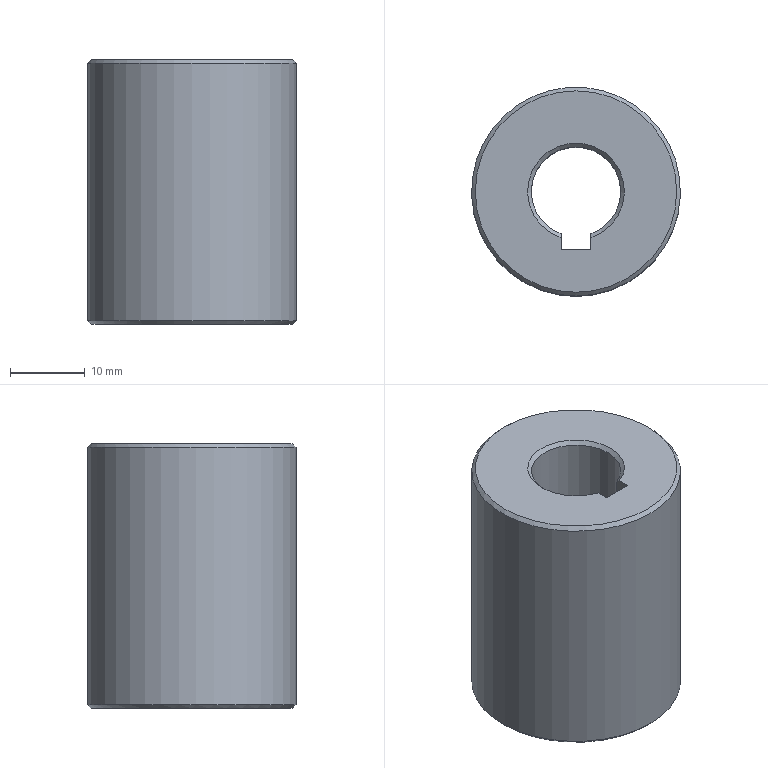Part | STEP file | 1 solid | 17 faces | box 28 x 28 x 35.5 mm | volume 17370 mm3 | cone 8 | plane 5 | cylinder 4 | commonest cylinder face diameters 3.242 x2 12 x1 28 x1
STEP:
#1=CARTESIAN_POINT('',(0.,0.,0.));
#2=DIRECTION('',(0.,0.,1.));
#3=DIRECTION('',(1.,0.,0.));
#4=AXIS2_PLACEMENT_3D('',#1,#2,#3);
#5=CARTESIAN_POINT('',(0.,-14.,0.5));
#6=VERTEX_POINT('',#5);
#7=CARTESIAN_POINT('',(0.,0.,0.5));
#8=DIRECTION('',(0.,0.,1.));
#9=DIRECTION('',(1.,0.,0.));
#10=AXIS2_PLACEMENT_3D('',#7,#8,#9);
#11=CIRCLE('',#10,14.);
#12=CARTESIAN_POINT('',(0.,0.,0.5));
#13=DIRECTION('',(0.,0.,1.));
#14=DIRECTION('',(0.,1.,0.));
#15=AXIS2_PLACEMENT_3D('',#12,#13,#14);
#16=CONICAL_SURFACE('',#15,14.,0.7854);
#17=CARTESIAN_POINT('',(-1.571,0.));
#18=DIRECTION('',(1.,0.));
#19=VECTOR('',#18,1.);
#20=LINE('',#17,#19);
#21=(GEOMETRIC_REPRESENTATION_CONTEXT(2)PARAMETRIC_REPRESENTATION_CONTEXT()REPRESENTATION_CONTEXT('',''));
#22=DEFINITIONAL_REPRESENTATION('',(#20),#21);
#23=PCURVE('',#16,#22);
#24=CARTESIAN_POINT('',(0.,0.,17.75));
#25=DIRECTION('',(0.,0.,-1.));
#26=DIRECTION('',(0.,-1.,0.));
#27=AXIS2_PLACEMENT_3D('',#24,#25,#26);
#28=CYLINDRICAL_SURFACE('',#27,14.);
#29=CARTESIAN_POINT('',(10.996,17.25));
#30=DIRECTION('',(-1.,0.));
#31=VECTOR('',#30,1.);
#32=LINE('',#29,#31);
#33=(GEOMETRIC_REPRESENTATION_CONTEXT(2)PARAMETRIC_REPRESENTATION_CONTEXT()REPRESENTATION_CONTEXT('',''));
#34=DEFINITIONAL_REPRESENTATION('',(#32),#33);
#35=PCURVE('',#28,#34);
#36=SURFACE_CURVE('',#11,(#23,#35),.PCURVE_S1.);
#37=EDGE_CURVE('',#6,#6,#36,.T.);
#38=ORIENTED_EDGE('',*,*,#37,.F.);
#39=CARTESIAN_POINT('',(0.,-13.5,0.));
#40=VERTEX_POINT('',#39);
#41=CARTESIAN_POINT('',(0.,-13.5,0.));
#42=CARTESIAN_POINT('',(0.,-14.,0.5));
#43=B_SPLINE_CURVE_WITH_KNOTS('',1,(#41,#42),.UNSPECIFIED.,.F.,.F.,(2,2),(-0.7071,0.),.PIECEWISE_BEZIER_KNOTS.);
#44=CARTESIAN_POINT('',(3.142,0.));
#45=DIRECTION('',(0.,1.));
#46=VECTOR('',#45,1.);
#47=LINE('',#44,#46);
#48=(GEOMETRIC_REPRESENTATION_CONTEXT(2)PARAMETRIC_REPRESENTATION_CONTEXT()REPRESENTATION_CONTEXT('',''));
#49=DEFINITIONAL_REPRESENTATION('',(#47),#48);
#50=PCURVE('',#16,#49);
#51=CARTESIAN_POINT('',(9.425,0.));
#52=DIRECTION('',(0.,1.));
#53=VECTOR('',#52,1.);
#54=LINE('',#51,#53);
#55=(GEOMETRIC_REPRESENTATION_CONTEXT(2)PARAMETRIC_REPRESENTATION_CONTEXT()REPRESENTATION_CONTEXT('',''));
#56=DEFINITIONAL_REPRESENTATION('',(#54),#55);
#57=PCURVE('',#16,#56);
#58=SEAM_CURVE('',#43,(#50,#57),.PCURVE_S1.);
#59=EDGE_CURVE('',#40,#6,#58,.T.);
#60=ORIENTED_EDGE('',*,*,#59,.F.);
#61=CARTESIAN_POINT('',(0.,0.,0.));
#62=DIRECTION('',(0.,0.,1.));
#63=DIRECTION('',(1.,0.,0.));
#64=AXIS2_PLACEMENT_3D('',#61,#62,#63);
#65=CIRCLE('',#64,13.5);
#66=CARTESIAN_POINT('',(-1.571,-0.5));
#67=DIRECTION('',(1.,0.));
#68=VECTOR('',#67,1.);
#69=LINE('',#66,#68);
#70=(GEOMETRIC_REPRESENTATION_CONTEXT(2)PARAMETRIC_REPRESENTATION_CONTEXT()REPRESENTATION_CONTEXT('',''));
#71=DEFINITIONAL_REPRESENTATION('',(#69),#70);
#72=PCURVE('',#16,#71);
#73=CARTESIAN_POINT('',(0.,10.,0.));
#74=DIRECTION('',(0.,0.,1.));
#75=DIRECTION('',(1.,0.,0.));
#76=AXIS2_PLACEMENT_3D('',#73,#74,#75);
#77=PLANE('',#76);
#78=CARTESIAN_POINT('',(0.,-10.));
#79=DIRECTION('',(1.,0.));
#80=AXIS2_PLACEMENT_2D('',#78,#79);
#81=CIRCLE('',#80,13.5);
#82=(GEOMETRIC_REPRESENTATION_CONTEXT(2)PARAMETRIC_REPRESENTATION_CONTEXT()REPRESENTATION_CONTEXT('',''));
#83=DEFINITIONAL_REPRESENTATION('',(#81),#82);
#84=PCURVE('',#77,#83);
#85=SURFACE_CURVE('',#65,(#72,#84),.PCURVE_S1.);
#86=EDGE_CURVE('',#40,#40,#85,.T.);
#87=ORIENTED_EDGE('',*,*,#86,.T.);
#88=ORIENTED_EDGE('',*,*,#59,.T.);
#89=EDGE_LOOP('',(#38,#60,#87,#88));
#90=FACE_BOUND('',#89,.T.);
#91=ADVANCED_FACE('',(#90),#16,.T.);
#92=CARTESIAN_POINT('',(0.,-14.,35.));
#93=VERTEX_POINT('',#92);
#94=CARTESIAN_POINT('',(0.,0.,35.));
#95=DIRECTION('',(0.,0.,-1.));
#96=DIRECTION('',(1.,0.,0.));
#97=AXIS2_PLACEMENT_3D('',#94,#95,#96);
#98=CIRCLE('',#97,14.);
#99=CARTESIAN_POINT('',(-1.571,-17.25));
#100=DIRECTION('',(1.,0.));
#101=VECTOR('',#100,1.);
#102=LINE('',#99,#101);
#103=(GEOMETRIC_REPRESENTATION_CONTEXT(2)PARAMETRIC_REPRESENTATION_CONTEXT()REPRESENTATION_CONTEXT('',''));
#104=DEFINITIONAL_REPRESENTATION('',(#102),#103);
#105=PCURVE('',#28,#104);
#106=CARTESIAN_POINT('',(0.,0.,35.));
#107=DIRECTION('',(0.,0.,-1.));
#108=DIRECTION('',(0.,-1.,0.));
#109=AXIS2_PLACEMENT_3D('',#106,#107,#108);
#110=CONICAL_SURFACE('',#109,14.,0.7854);
#111=CARTESIAN_POINT('',(-1.571,0.));
#112=DIRECTION('',(1.,0.));
#113=VECTOR('',#112,1.);
#114=LINE('',#111,#113);
#115=(GEOMETRIC_REPRESENTATION_CONTEXT(2)PARAMETRIC_REPRESENTATION_CONTEXT()REPRESENTATION_CONTEXT('',''));
#116=DEFINITIONAL_REPRESENTATION('',(#114),#115);
#117=PCURVE('',#110,#116);
#118=SURFACE_CURVE('',#98,(#105,#117),.PCURVE_S1.);
#119=EDGE_CURVE('',#93,#93,#118,.T.);
#120=ORIENTED_EDGE('',*,*,#119,.T.);
#121=CARTESIAN_POINT('',(0.,-14.,35.));
#122=CARTESIAN_POINT('',(0.,-14.,0.5));
#123=B_SPLINE_CURVE_WITH_KNOTS('',1,(#121,#122),.UNSPECIFIED.,.F.,.F.,(2,2),(-17.25,17.25),.PIECEWISE_BEZIER_KNOTS.);
#124=CARTESIAN_POINT('',(6.283,0.));
#125=DIRECTION('',(0.,1.));
#126=VECTOR('',#125,1.);
#127=LINE('',#124,#126);
#128=(GEOMETRIC_REPRESENTATION_CONTEXT(2)PARAMETRIC_REPRESENTATION_CONTEXT()REPRESENTATION_CONTEXT('',''));
#129=DEFINITIONAL_REPRESENTATION('',(#127),#128);
#130=PCURVE('',#28,#129);
#131=CARTESIAN_POINT('',(0.,0.));
#132=DIRECTION('',(0.,1.));
#133=VECTOR('',#132,1.);
#134=LINE('',#131,#133);
#135=(GEOMETRIC_REPRESENTATION_CONTEXT(2)PARAMETRIC_REPRESENTATION_CONTEXT()REPRESENTATION_CONTEXT('',''));
#136=DEFINITIONAL_REPRESENTATION('',(#134),#135);
#137=PCURVE('',#28,#136);
#138=SEAM_CURVE('',#123,(#130,#137),.PCURVE_S1.);
#139=EDGE_CURVE('',#93,#6,#138,.T.);
#140=ORIENTED_EDGE('',*,*,#139,.T.);
#141=ORIENTED_EDGE('',*,*,#37,.T.);
#142=ORIENTED_EDGE('',*,*,#139,.F.);
#143=EDGE_LOOP('',(#120,#140,#141,#142));
#144=FACE_BOUND('',#143,.T.);
#145=ADVANCED_FACE('',(#144),#28,.T.);
#146=ORIENTED_EDGE('',*,*,#86,.F.);
#147=EDGE_LOOP('',(#146));
#148=FACE_BOUND('',#147,.T.);
#149=CARTESIAN_POINT('',(-2.,-6.185,0.));
#150=VERTEX_POINT('',#149);
#151=CARTESIAN_POINT('',(2.,-6.185,0.));
#152=VERTEX_POINT('',#151);
#153=CARTESIAN_POINT('',(0.,0.,0.));
#154=DIRECTION('',(0.,0.,-1.));
#155=DIRECTION('',(0.3077,-0.9515,0.));
#156=AXIS2_PLACEMENT_3D('',#153,#154,#155);
#157=CIRCLE('',#156,6.5);
#158=CARTESIAN_POINT('',(2.,-16.185));
#159=CARTESIAN_POINT('',(-8.712,-19.649));
#160=CARTESIAN_POINT('',(-6.356,-8.64));
#161=CARTESIAN_POINT('',(-4.,2.369));
#162=CARTESIAN_POINT('',(4.356,-5.176));
#163=CARTESIAN_POINT('',(12.712,-12.721));
#164=CARTESIAN_POINT('',(2.,-16.185));
#165=(BOUNDED_CURVE()B_SPLINE_CURVE(2,(#158,#159,#160,#161,#162,#163,#164),.UNSPECIFIED.,.T.,.F.)B_SPLINE_CURVE_WITH_KNOTS((1,2,2,2,2,1),(-2.094,0.,2.094,4.189,6.283,8.378),.UNSPECIFIED.)CURVE()GEOMETRIC_REPRESENTATION_ITEM()RATIONAL_B_SPLINE_CURVE((1.,0.5,1.,0.5,1.,0.5,1.))REPRESENTATION_ITEM(''));
#166=(GEOMETRIC_REPRESENTATION_CONTEXT(2)PARAMETRIC_REPRESENTATION_CONTEXT()REPRESENTATION_CONTEXT('',''));
#167=DEFINITIONAL_REPRESENTATION('',(#165),#166);
#168=PCURVE('',#77,#167);
#169=CARTESIAN_POINT('',(0.,0.,0.));
#170=DIRECTION('',(0.,0.,-1.));
#171=DIRECTION('',(0.,1.,0.));
#172=AXIS2_PLACEMENT_3D('',#169,#170,#171);
#173=CONICAL_SURFACE('',#172,6.5,0.7854);
#174=CARTESIAN_POINT('',(-3.454,0.));
#175=DIRECTION('',(1.,0.));
#176=VECTOR('',#175,1.);
#177=LINE('',#174,#176);
#178=(GEOMETRIC_REPRESENTATION_CONTEXT(2)PARAMETRIC_REPRESENTATION_CONTEXT()REPRESENTATION_CONTEXT('',''));
#179=DEFINITIONAL_REPRESENTATION('',(#177),#178);
#180=PCURVE('',#173,#179);
#181=SURFACE_CURVE('',#157,(#168,#180),.PCURVE_S1.);
#182=EDGE_CURVE('',#150,#152,#181,.T.);
#183=ORIENTED_EDGE('',*,*,#182,.F.);
#184=CARTESIAN_POINT('',(-2.,-7.8,0.));
#185=VERTEX_POINT('',#184);
#186=CARTESIAN_POINT('',(-2.,-6.185,0.));
#187=DIRECTION('',(0.,-1.,0.));
#188=VECTOR('',#187,1.);
#189=LINE('',#186,#188);
#190=CARTESIAN_POINT('',(-2.,-16.185));
#191=DIRECTION('',(0.,-1.));
#192=VECTOR('',#191,1.);
#193=LINE('',#190,#192);
#194=(GEOMETRIC_REPRESENTATION_CONTEXT(2)PARAMETRIC_REPRESENTATION_CONTEXT()REPRESENTATION_CONTEXT('',''));
#195=DEFINITIONAL_REPRESENTATION('',(#193),#194);
#196=PCURVE('',#77,#195);
#197=CARTESIAN_POINT('',(-2.,-7.8,0.));
#198=DIRECTION('',(-1.,0.,0.));
#199=DIRECTION('',(0.,0.,1.));
#200=AXIS2_PLACEMENT_3D('',#197,#198,#199);
#201=PLANE('',#200);
#202=CARTESIAN_POINT('',(0.,1.615));
#203=DIRECTION('',(0.,-1.));
#204=VECTOR('',#203,1.);
#205=LINE('',#202,#204);
#206=(GEOMETRIC_REPRESENTATION_CONTEXT(2)PARAMETRIC_REPRESENTATION_CONTEXT()REPRESENTATION_CONTEXT('',''));
#207=DEFINITIONAL_REPRESENTATION('',(#205),#206);
#208=PCURVE('',#201,#207);
#209=SURFACE_CURVE('',#189,(#196,#208),.PCURVE_S1.);
#210=EDGE_CURVE('',#150,#185,#209,.T.);
#211=ORIENTED_EDGE('',*,*,#210,.T.);
#212=CARTESIAN_POINT('',(2.,-7.8,0.));
#213=VERTEX_POINT('',#212);
#214=CARTESIAN_POINT('',(-2.,-7.8,0.));
#215=DIRECTION('',(1.,0.,0.));
#216=VECTOR('',#215,1.);
#217=LINE('',#214,#216);
#218=CARTESIAN_POINT('',(-2.,-17.8));
#219=DIRECTION('',(1.,0.));
#220=VECTOR('',#219,1.);
#221=LINE('',#218,#220);
#222=(GEOMETRIC_REPRESENTATION_CONTEXT(2)PARAMETRIC_REPRESENTATION_CONTEXT()REPRESENTATION_CONTEXT('',''));
#223=DEFINITIONAL_REPRESENTATION('',(#221),#222);
#224=PCURVE('',#77,#223);
#225=CARTESIAN_POINT('',(2.,-7.8,0.));
#226=DIRECTION('',(0.,-1.,0.));
#227=DIRECTION('',(0.,0.,-1.));
#228=AXIS2_PLACEMENT_3D('',#225,#226,#227);
#229=PLANE('',#228);
#230=CARTESIAN_POINT('',(0.,-4.));
#231=DIRECTION('',(0.,1.));
#232=VECTOR('',#231,1.);
#233=LINE('',#230,#232);
#234=(GEOMETRIC_REPRESENTATION_CONTEXT(2)PARAMETRIC_REPRESENTATION_CONTEXT()REPRESENTATION_CONTEXT('',''));
#235=DEFINITIONAL_REPRESENTATION('',(#233),#234);
#236=PCURVE('',#229,#235);
#237=SURFACE_CURVE('',#217,(#224,#236),.PCURVE_S1.);
#238=EDGE_CURVE('',#185,#213,#237,.T.);
#239=ORIENTED_EDGE('',*,*,#238,.T.);
#240=CARTESIAN_POINT('',(2.,-7.8,0.));
#241=DIRECTION('',(0.,1.,0.));
#242=VECTOR('',#241,1.);
#243=LINE('',#240,#242);
#244=CARTESIAN_POINT('',(2.,-17.8));
#245=DIRECTION('',(0.,1.));
#246=VECTOR('',#245,1.);
#247=LINE('',#244,#246);
#248=(GEOMETRIC_REPRESENTATION_CONTEXT(2)PARAMETRIC_REPRESENTATION_CONTEXT()REPRESENTATION_CONTEXT('',''));
#249=DEFINITIONAL_REPRESENTATION('',(#247),#248);
#250=PCURVE('',#77,#249);
#251=CARTESIAN_POINT('',(2.,0.,0.));
#252=DIRECTION('',(1.,0.,0.));
#253=DIRECTION('',(0.,0.,-1.));
#254=AXIS2_PLACEMENT_3D('',#251,#252,#253);
#255=PLANE('',#254);
#256=CARTESIAN_POINT('',(0.,-7.8));
#257=DIRECTION('',(0.,1.));
#258=VECTOR('',#257,1.);
#259=LINE('',#256,#258);
#260=(GEOMETRIC_REPRESENTATION_CONTEXT(2)PARAMETRIC_REPRESENTATION_CONTEXT()REPRESENTATION_CONTEXT('',''));
#261=DEFINITIONAL_REPRESENTATION('',(#259),#260);
#262=PCURVE('',#255,#261);
#263=SURFACE_CURVE('',#243,(#250,#262),.PCURVE_S1.);
#264=EDGE_CURVE('',#213,#152,#263,.T.);
#265=ORIENTED_EDGE('',*,*,#264,.T.);
#266=EDGE_LOOP('',(#183,#211,#239,#265));
#267=FACE_BOUND('',#266,.T.);
#268=CARTESIAN_POINT('',(8.,0.,0.));
#269=VERTEX_POINT('',#268);
#270=CARTESIAN_POINT('',(10.,0.,0.));
#271=DIRECTION('',(0.,0.,-1.));
#272=DIRECTION('',(1.,0.,0.));
#273=AXIS2_PLACEMENT_3D('',#270,#271,#272);
#274=CIRCLE('',#273,2.);
#275=CARTESIAN_POINT('',(12.,-10.));
#276=CARTESIAN_POINT('',(12.,-13.464));
#277=CARTESIAN_POINT('',(9.,-11.732));
#278=CARTESIAN_POINT('',(6.,-10.));
#279=CARTESIAN_POINT('',(9.,-8.268));
#280=CARTESIAN_POINT('',(12.,-6.536));
#281=CARTESIAN_POINT('',(12.,-10.));
#282=(BOUNDED_CURVE()B_SPLINE_CURVE(2,(#275,#276,#277,#278,#279,#280,#281),.UNSPECIFIED.,.T.,.F.)B_SPLINE_CURVE_WITH_KNOTS((1,2,2,2,2,1),(-2.094,0.,2.094,4.189,6.283,8.378),.UNSPECIFIED.)CURVE()GEOMETRIC_REPRESENTATION_ITEM()RATIONAL_B_SPLINE_CURVE((1.,0.5,1.,0.5,1.,0.5,1.))REPRESENTATION_ITEM(''));
#283=(GEOMETRIC_REPRESENTATION_CONTEXT(2)PARAMETRIC_REPRESENTATION_CONTEXT()REPRESENTATION_CONTEXT('',''));
#284=DEFINITIONAL_REPRESENTATION('',(#282),#283);
#285=PCURVE('',#77,#284);
#286=CARTESIAN_POINT('',(10.,0.,0.));
#287=DIRECTION('',(0.,0.,-1.));
#288=DIRECTION('',(-1.,0.,0.));
#289=AXIS2_PLACEMENT_3D('',#286,#287,#288);
#290=CONICAL_SURFACE('',#289,2.,0.7854);
#291=CARTESIAN_POINT('',(-3.142,0.));
#292=DIRECTION('',(1.,0.));
#293=VECTOR('',#292,1.);
#294=LINE('',#291,#293);
#295=(GEOMETRIC_REPRESENTATION_CONTEXT(2)PARAMETRIC_REPRESENTATION_CONTEXT()REPRESENTATION_CONTEXT('',''));
#296=DEFINITIONAL_REPRESENTATION('',(#294),#295);
#297=PCURVE('',#290,#296);
#298=SURFACE_CURVE('',#274,(#285,#297),.PCURVE_S1.);
#299=EDGE_CURVE('',#269,#269,#298,.T.);
#300=ORIENTED_EDGE('',*,*,#299,.F.);
#301=EDGE_LOOP('',(#300));
#302=FACE_BOUND('',#301,.T.);
#303=CARTESIAN_POINT('',(-12.,0.,0.));
#304=VERTEX_POINT('',#303);
#305=CARTESIAN_POINT('',(-10.,0.,0.));
#306=DIRECTION('',(0.,0.,-1.));
#307=DIRECTION('',(1.,0.,0.));
#308=AXIS2_PLACEMENT_3D('',#305,#306,#307);
#309=CIRCLE('',#308,2.);
#310=CARTESIAN_POINT('',(-8.,-10.));
#311=CARTESIAN_POINT('',(-8.,-13.464));
#312=CARTESIAN_POINT('',(-11.,-11.732));
#313=CARTESIAN_POINT('',(-14.,-10.));
#314=CARTESIAN_POINT('',(-11.,-8.268));
#315=CARTESIAN_POINT('',(-8.,-6.536));
#316=CARTESIAN_POINT('',(-8.,-10.));
#317=(BOUNDED_CURVE()B_SPLINE_CURVE(2,(#310,#311,#312,#313,#314,#315,#316),.UNSPECIFIED.,.T.,.F.)B_SPLINE_CURVE_WITH_KNOTS((1,2,2,2,2,1),(-2.094,0.,2.094,4.189,6.283,8.378),.UNSPECIFIED.)CURVE()GEOMETRIC_REPRESENTATION_ITEM()RATIONAL_B_SPLINE_CURVE((1.,0.5,1.,0.5,1.,0.5,1.))REPRESENTATION_ITEM(''));
#318=(GEOMETRIC_REPRESENTATION_CONTEXT(2)PARAMETRIC_REPRESENTATION_CONTEXT()REPRESENTATION_CONTEXT('',''));
#319=DEFINITIONAL_REPRESENTATION('',(#317),#318);
#320=PCURVE('',#77,#319);
#321=CARTESIAN_POINT('',(-10.,0.,0.));
#322=DIRECTION('',(0.,0.,-1.));
#323=DIRECTION('',(-1.,0.,0.));
#324=AXIS2_PLACEMENT_3D('',#321,#322,#323);
#325=CONICAL_SURFACE('',#324,2.,0.7854);
#326=CARTESIAN_POINT('',(-3.142,0.));
#327=DIRECTION('',(1.,0.));
#328=VECTOR('',#327,1.);
#329=LINE('',#326,#328);
#330=(GEOMETRIC_REPRESENTATION_CONTEXT(2)PARAMETRIC_REPRESENTATION_CONTEXT()REPRESENTATION_CONTEXT('',''));
#331=DEFINITIONAL_REPRESENTATION('',(#329),#330);
#332=PCURVE('',#325,#331);
#333=SURFACE_CURVE('',#309,(#320,#332),.PCURVE_S1.);
#334=EDGE_CURVE('',#304,#304,#333,.T.);
#335=ORIENTED_EDGE('',*,*,#334,.F.);
#336=EDGE_LOOP('',(#335));
#337=FACE_BOUND('',#336,.T.);
#338=ADVANCED_FACE('',(#148,#267,#302,#337),#77,.F.);
#339=CARTESIAN_POINT('',(0.,-13.5,35.5));
#340=VERTEX_POINT('',#339);
#341=CARTESIAN_POINT('',(0.,0.,35.5));
#342=DIRECTION('',(0.,0.,-1.));
#343=DIRECTION('',(1.,0.,0.));
#344=AXIS2_PLACEMENT_3D('',#341,#342,#343);
#345=CIRCLE('',#344,13.5);
#346=CARTESIAN_POINT('',(-1.571,-0.5));
#347=DIRECTION('',(1.,0.));
#348=VECTOR('',#347,1.);
#349=LINE('',#346,#348);
#350=(GEOMETRIC_REPRESENTATION_CONTEXT(2)PARAMETRIC_REPRESENTATION_CONTEXT()REPRESENTATION_CONTEXT('',''));
#351=DEFINITIONAL_REPRESENTATION('',(#349),#350);
#352=PCURVE('',#110,#351);
#353=CARTESIAN_POINT('',(0.,10.,35.5));
#354=DIRECTION('',(0.,0.,1.));
#355=DIRECTION('',(1.,0.,0.));
#356=AXIS2_PLACEMENT_3D('',#353,#354,#355);
#357=PLANE('',#356);
#358=CARTESIAN_POINT('',(13.5,-10.));
#359=CARTESIAN_POINT('',(13.5,-33.383));
#360=CARTESIAN_POINT('',(-6.75,-21.691));
#361=CARTESIAN_POINT('',(-27.,-10.));
#362=CARTESIAN_POINT('',(-6.75,1.691));
#363=CARTESIAN_POINT('',(13.5,13.383));
#364=CARTESIAN_POINT('',(13.5,-10.));
#365=(BOUNDED_CURVE()B_SPLINE_CURVE(2,(#358,#359,#360,#361,#362,#363,#364),.UNSPECIFIED.,.T.,.F.)B_SPLINE_CURVE_WITH_KNOTS((1,2,2,2,2,1),(-2.094,0.,2.094,4.189,6.283,8.378),.UNSPECIFIED.)CURVE()GEOMETRIC_REPRESENTATION_ITEM()RATIONAL_B_SPLINE_CURVE((1.,0.5,1.,0.5,1.,0.5,1.))REPRESENTATION_ITEM(''));
#366=(GEOMETRIC_REPRESENTATION_CONTEXT(2)PARAMETRIC_REPRESENTATION_CONTEXT()REPRESENTATION_CONTEXT('',''));
#367=DEFINITIONAL_REPRESENTATION('',(#365),#366);
#368=PCURVE('',#357,#367);
#369=SURFACE_CURVE('',#345,(#352,#368),.PCURVE_S1.);
#370=EDGE_CURVE('',#340,#340,#369,.T.);
#371=ORIENTED_EDGE('',*,*,#370,.T.);
#372=CARTESIAN_POINT('',(0.,-13.5,35.5));
#373=CARTESIAN_POINT('',(0.,-14.,35.));
#374=B_SPLINE_CURVE_WITH_KNOTS('',1,(#372,#373),.UNSPECIFIED.,.F.,.F.,(2,2),(-0.7071,0.),.PIECEWISE_BEZIER_KNOTS.);
#375=CARTESIAN_POINT('',(6.283,0.));
#376=DIRECTION('',(0.,1.));
#377=VECTOR('',#376,1.);
#378=LINE('',#375,#377);
#379=(GEOMETRIC_REPRESENTATION_CONTEXT(2)PARAMETRIC_REPRESENTATION_CONTEXT()REPRESENTATION_CONTEXT('',''));
#380=DEFINITIONAL_REPRESENTATION('',(#378),#379);
#381=PCURVE('',#110,#380);
#382=CARTESIAN_POINT('',(0.,0.));
#383=DIRECTION('',(0.,1.));
#384=VECTOR('',#383,1.);
#385=LINE('',#382,#384);
#386=(GEOMETRIC_REPRESENTATION_CONTEXT(2)PARAMETRIC_REPRESENTATION_CONTEXT()REPRESENTATION_CONTEXT('',''));
#387=DEFINITIONAL_REPRESENTATION('',(#385),#386);
#388=PCURVE('',#110,#387);
#389=SEAM_CURVE('',#374,(#381,#388),.PCURVE_S1.);
#390=EDGE_CURVE('',#340,#93,#389,.T.);
#391=ORIENTED_EDGE('',*,*,#390,.T.);
#392=ORIENTED_EDGE('',*,*,#119,.F.);
#393=ORIENTED_EDGE('',*,*,#390,.F.);
#394=EDGE_LOOP('',(#371,#391,#392,#393));
#395=FACE_BOUND('',#394,.T.);
#396=ADVANCED_FACE('',(#395),#110,.T.);
#397=CARTESIAN_POINT('',(-2.,-5.657,0.5));
#398=VERTEX_POINT('',#397);
#399=CARTESIAN_POINT('',(-2.,7.228,-1.));
#400=CARTESIAN_POINT('',(-2.,0.,5.967));
#401=CARTESIAN_POINT('',(-2.,-7.228,-1.));
#402=(BOUNDED_CURVE()B_SPLINE_CURVE(2,(#399,#400,#401),.UNSPECIFIED.,.F.,.F.)B_SPLINE_CURVE_WITH_KNOTS((3,3),(0.,1.817),.PIECEWISE_BEZIER_KNOTS.)CURVE()GEOMETRIC_REPRESENTATION_ITEM()RATIONAL_B_SPLINE_CURVE((1.,3.75,1.))REPRESENTATION_ITEM(''));
#403=CARTESIAN_POINT('',(-2.802,-0.5));
#404=CARTESIAN_POINT('',(-2.802,-0.493));
#405=CARTESIAN_POINT('',(-2.803,-0.4789));
#406=CARTESIAN_POINT('',(-2.804,-0.4576));
#407=CARTESIAN_POINT('',(-2.805,-0.4361));
#408=CARTESIAN_POINT('',(-2.807,-0.4146));
#409=CARTESIAN_POINT('',(-2.808,-0.3928));
#410=CARTESIAN_POINT('',(-2.809,-0.371));
#411=CARTESIAN_POINT('',(-2.81,-0.349));
#412=CARTESIAN_POINT('',(-2.812,-0.3268));
#413=CARTESIAN_POINT('',(-2.813,-0.3045));
#414=CARTESIAN_POINT('',(-2.814,-0.282));
#415=CARTESIAN_POINT('',(-2.815,-0.2594));
#416=CARTESIAN_POINT('',(-2.817,-0.2366));
#417=CARTESIAN_POINT('',(-2.818,-0.2137));
#418=CARTESIAN_POINT('',(-2.819,-0.1906));
#419=CARTESIAN_POINT('',(-2.82,-0.1673));
#420=CARTESIAN_POINT('',(-2.821,-0.1439));
#421=CARTESIAN_POINT('',(-2.823,-0.1204));
#422=CARTESIAN_POINT('',(-2.824,-0.09664));
#423=CARTESIAN_POINT('',(-2.825,-0.07274));
#424=CARTESIAN_POINT('',(-2.826,-0.04867));
#425=CARTESIAN_POINT('',(-2.828,-0.02444));
#426=CARTESIAN_POINT('',(-2.828,-0.008164));
#427=CARTESIAN_POINT('',(-2.829,0.));
#428=B_SPLINE_CURVE_WITH_KNOTS('',3,(#403,#404,#405,#406,#407,#408,#409,#410,#411,#412,#413,#414,#415,#416,#417,#418,#419,#420,#421,#422,#423,#424,#425,#426,#427),.UNSPECIFIED.,.F.,.F.,(4,1,1,1,1,1,1,1,1,1,1,1,1,1,1,1,1,1,1,1,1,1,4),(1.752,1.754,1.755,1.756,1.757,1.758,1.759,1.76,1.761,1.762,1.764,1.765,1.766,1.767,1.768,1.769,1.77,1.771,1.772,1.774,1.775,1.776,1.777),.QUASI_UNIFORM_KNOTS.);
#429=(GEOMETRIC_REPRESENTATION_CONTEXT(2)PARAMETRIC_REPRESENTATION_CONTEXT()REPRESENTATION_CONTEXT('',''));
#430=DEFINITIONAL_REPRESENTATION('',(#428),#429);
#431=PCURVE('',#173,#430);
#432=CARTESIAN_POINT('',(-1.,15.028));
#433=CARTESIAN_POINT('',(5.967,7.8));
#434=CARTESIAN_POINT('',(-1.,0.5716));
#435=(BOUNDED_CURVE()B_SPLINE_CURVE(2,(#432,#433,#434),.UNSPECIFIED.,.F.,.F.)B_SPLINE_CURVE_WITH_KNOTS((3,3),(0.,1.817),.PIECEWISE_BEZIER_KNOTS.)CURVE()GEOMETRIC_REPRESENTATION_ITEM()RATIONAL_B_SPLINE_CURVE((1.,3.75,1.))REPRESENTATION_ITEM(''));
#436=(GEOMETRIC_REPRESENTATION_CONTEXT(2)PARAMETRIC_REPRESENTATION_CONTEXT()REPRESENTATION_CONTEXT('',''));
#437=DEFINITIONAL_REPRESENTATION('',(#435),#436);
#438=PCURVE('',#201,#437);
#439=SURFACE_CURVE('',#402,(#431,#438),.PCURVE_S1.);
#440=EDGE_CURVE('',#398,#150,#439,.T.);
#441=ORIENTED_EDGE('',*,*,#440,.F.);
#442=CARTESIAN_POINT('',(2.,-5.657,0.5));
#443=VERTEX_POINT('',#442);
#444=CARTESIAN_POINT('',(0.,0.,0.5));
#445=DIRECTION('',(0.,0.,-1.));
#446=DIRECTION('',(1.,0.,0.));
#447=AXIS2_PLACEMENT_3D('',#444,#445,#446);
#448=CIRCLE('',#447,6.);
#449=CARTESIAN_POINT('',(-4.712,-0.5));
#450=DIRECTION('',(1.,0.));
#451=VECTOR('',#450,1.);
#452=LINE('',#449,#451);
#453=(GEOMETRIC_REPRESENTATION_CONTEXT(2)PARAMETRIC_REPRESENTATION_CONTEXT()REPRESENTATION_CONTEXT('',''));
#454=DEFINITIONAL_REPRESENTATION('',(#452),#453);
#455=PCURVE('',#173,#454);
#456=CARTESIAN_POINT('',(0.,0.,17.75));
#457=DIRECTION('',(0.,0.,-1.));
#458=DIRECTION('',(0.,1.,0.));
#459=AXIS2_PLACEMENT_3D('',#456,#457,#458);
#460=CYLINDRICAL_SURFACE('',#459,6.);
#461=CARTESIAN_POINT('',(-4.712,17.25));
#462=DIRECTION('',(1.,0.));
#463=VECTOR('',#462,1.);
#464=LINE('',#461,#463);
#465=(GEOMETRIC_REPRESENTATION_CONTEXT(2)PARAMETRIC_REPRESENTATION_CONTEXT()REPRESENTATION_CONTEXT('',''));
#466=DEFINITIONAL_REPRESENTATION('',(#464),#465);
#467=PCURVE('',#460,#466);
#468=SURFACE_CURVE('',#448,(#455,#467),.PCURVE_S1.);
#469=EDGE_CURVE('',#398,#443,#468,.T.);
#470=ORIENTED_EDGE('',*,*,#469,.T.);
#471=CARTESIAN_POINT('',(2.,-7.228,-1.));
#472=CARTESIAN_POINT('',(2.,0.,5.967));
#473=CARTESIAN_POINT('',(2.,7.228,-1.));
#474=(BOUNDED_CURVE()B_SPLINE_CURVE(2,(#471,#472,#473),.UNSPECIFIED.,.F.,.F.)B_SPLINE_CURVE_WITH_KNOTS((3,3),(0.,1.817),.PIECEWISE_BEZIER_KNOTS.)CURVE()GEOMETRIC_REPRESENTATION_ITEM()RATIONAL_B_SPLINE_CURVE((1.,3.75,1.))REPRESENTATION_ITEM(''));
#475=CARTESIAN_POINT('',(2.829,0.));
#476=CARTESIAN_POINT('',(2.828,-0.008164));
#477=CARTESIAN_POINT('',(2.828,-0.02444));
#478=CARTESIAN_POINT('',(2.826,-0.04867));
#479=CARTESIAN_POINT('',(2.825,-0.07274));
#480=CARTESIAN_POINT('',(2.824,-0.09664));
#481=CARTESIAN_POINT('',(2.823,-0.1204));
#482=CARTESIAN_POINT('',(2.821,-0.1439));
#483=CARTESIAN_POINT('',(2.82,-0.1673));
#484=CARTESIAN_POINT('',(2.819,-0.1906));
#485=CARTESIAN_POINT('',(2.818,-0.2137));
#486=CARTESIAN_POINT('',(2.817,-0.2366));
#487=CARTESIAN_POINT('',(2.815,-0.2594));
#488=CARTESIAN_POINT('',(2.814,-0.282));
#489=CARTESIAN_POINT('',(2.813,-0.3045));
#490=CARTESIAN_POINT('',(2.812,-0.3268));
#491=CARTESIAN_POINT('',(2.81,-0.349));
#492=CARTESIAN_POINT('',(2.809,-0.371));
#493=CARTESIAN_POINT('',(2.808,-0.3928));
#494=CARTESIAN_POINT('',(2.807,-0.4146));
#495=CARTESIAN_POINT('',(2.805,-0.4361));
#496=CARTESIAN_POINT('',(2.804,-0.4576));
#497=CARTESIAN_POINT('',(2.803,-0.4789));
#498=CARTESIAN_POINT('',(2.802,-0.493));
#499=CARTESIAN_POINT('',(2.802,-0.5));
#500=B_SPLINE_CURVE_WITH_KNOTS('',3,(#475,#476,#477,#478,#479,#480,#481,#482,#483,#484,#485,#486,#487,#488,#489,#490,#491,#492,#493,#494,#495,#496,#497,#498,#499),.UNSPECIFIED.,.F.,.F.,(4,1,1,1,1,1,1,1,1,1,1,1,1,1,1,1,1,1,1,1,1,1,4),(0.03973,0.04084,0.04195,0.04306,0.04418,0.04529,0.0464,0.04751,0.04863,0.04974,0.05085,0.05196,0.05307,0.05419,0.0553,0.05641,0.05752,0.05864,0.05975,0.06086,0.06197,0.06309,0.0642),.QUASI_UNIFORM_KNOTS.);
#501=(GEOMETRIC_REPRESENTATION_CONTEXT(2)PARAMETRIC_REPRESENTATION_CONTEXT()REPRESENTATION_CONTEXT('',''));
#502=DEFINITIONAL_REPRESENTATION('',(#500),#501);
#503=PCURVE('',#173,#502);
#504=CARTESIAN_POINT('',(1.,-7.228));
#505=CARTESIAN_POINT('',(-5.967,0.));
#506=CARTESIAN_POINT('',(1.,7.228));
#507=(BOUNDED_CURVE()B_SPLINE_CURVE(2,(#504,#505,#506),.UNSPECIFIED.,.F.,.F.)B_SPLINE_CURVE_WITH_KNOTS((3,3),(0.,1.817),.PIECEWISE_BEZIER_KNOTS.)CURVE()GEOMETRIC_REPRESENTATION_ITEM()RATIONAL_B_SPLINE_CURVE((1.,3.75,1.))REPRESENTATION_ITEM(''));
#508=(GEOMETRIC_REPRESENTATION_CONTEXT(2)PARAMETRIC_REPRESENTATION_CONTEXT()REPRESENTATION_CONTEXT('',''));
#509=DEFINITIONAL_REPRESENTATION('',(#507),#508);
#510=PCURVE('',#255,#509);
#511=SURFACE_CURVE('',#474,(#503,#510),.PCURVE_S1.);
#512=EDGE_CURVE('',#152,#443,#511,.T.);
#513=ORIENTED_EDGE('',*,*,#512,.F.);
#514=ORIENTED_EDGE('',*,*,#182,.F.);
#515=EDGE_LOOP('',(#441,#470,#513,#514));
#516=FACE_BOUND('',#515,.F.);
#517=ADVANCED_FACE('',(#516),#173,.F.);
#518=CARTESIAN_POINT('',(-2.,-6.185,35.5));
#519=VERTEX_POINT('',#518);
#520=CARTESIAN_POINT('',(-2.,-7.8,35.5));
#521=VERTEX_POINT('',#520);
#522=CARTESIAN_POINT('',(-2.,-6.185,35.5));
#523=DIRECTION('',(0.,-1.,0.));
#524=VECTOR('',#523,1.);
#525=LINE('',#522,#524);
#526=CARTESIAN_POINT('',(35.5,1.615));
#527=DIRECTION('',(0.,-1.));
#528=VECTOR('',#527,1.);
#529=LINE('',#526,#528);
#530=(GEOMETRIC_REPRESENTATION_CONTEXT(2)PARAMETRIC_REPRESENTATION_CONTEXT()REPRESENTATION_CONTEXT('',''));
#531=DEFINITIONAL_REPRESENTATION('',(#529),#530);
#532=PCURVE('',#201,#531);
#533=CARTESIAN_POINT('',(-2.,-16.185));
#534=DIRECTION('',(0.,-1.));
#535=VECTOR('',#534,1.);
#536=LINE('',#533,#535);
#537=(GEOMETRIC_REPRESENTATION_CONTEXT(2)PARAMETRIC_REPRESENTATION_CONTEXT()REPRESENTATION_CONTEXT('',''));
#538=DEFINITIONAL_REPRESENTATION('',(#536),#537);
#539=PCURVE('',#357,#538);
#540=SURFACE_CURVE('',#525,(#532,#539),.PCURVE_S1.);
#541=EDGE_CURVE('',#519,#521,#540,.T.);
#542=ORIENTED_EDGE('',*,*,#541,.T.);
#543=CARTESIAN_POINT('',(-2.,-7.8,0.));
#544=DIRECTION('',(0.,0.,1.));
#545=VECTOR('',#544,1.);
#546=LINE('',#543,#545);
#547=CARTESIAN_POINT('',(0.,0.));
#548=DIRECTION('',(1.,0.));
#549=VECTOR('',#548,1.);
#550=LINE('',#547,#549);
#551=(GEOMETRIC_REPRESENTATION_CONTEXT(2)PARAMETRIC_REPRESENTATION_CONTEXT()REPRESENTATION_CONTEXT('',''));
#552=DEFINITIONAL_REPRESENTATION('',(#550),#551);
#553=PCURVE('',#201,#552);
#554=CARTESIAN_POINT('',(0.,-4.));
#555=DIRECTION('',(-1.,0.));
#556=VECTOR('',#555,1.);
#557=LINE('',#554,#556);
#558=(GEOMETRIC_REPRESENTATION_CONTEXT(2)PARAMETRIC_REPRESENTATION_CONTEXT()REPRESENTATION_CONTEXT('',''));
#559=DEFINITIONAL_REPRESENTATION('',(#557),#558);
#560=PCURVE('',#229,#559);
#561=SURFACE_CURVE('',#546,(#553,#560),.PCURVE_S1.);
#562=EDGE_CURVE('',#185,#521,#561,.T.);
#563=ORIENTED_EDGE('',*,*,#562,.F.);
#564=ORIENTED_EDGE('',*,*,#210,.F.);
#565=ORIENTED_EDGE('',*,*,#440,.F.);
#566=CARTESIAN_POINT('',(-2.,-5.657,35.));
#567=VERTEX_POINT('',#566);
#568=CARTESIAN_POINT('',(-2.,-5.657,35.));
#569=DIRECTION('',(0.,0.,-1.));
#570=VECTOR('',#569,1.);
#571=LINE('',#568,#570);
#572=CARTESIAN_POINT('',(35.,2.143));
#573=DIRECTION('',(-1.,0.));
#574=VECTOR('',#573,1.);
#575=LINE('',#572,#574);
#576=(GEOMETRIC_REPRESENTATION_CONTEXT(2)PARAMETRIC_REPRESENTATION_CONTEXT()REPRESENTATION_CONTEXT('',''));
#577=DEFINITIONAL_REPRESENTATION('',(#575),#576);
#578=PCURVE('',#201,#577);
#579=CARTESIAN_POINT('',(-2.802,-17.25));
#580=DIRECTION('',(0.,1.));
#581=VECTOR('',#580,1.);
#582=LINE('',#579,#581);
#583=(GEOMETRIC_REPRESENTATION_CONTEXT(2)PARAMETRIC_REPRESENTATION_CONTEXT()REPRESENTATION_CONTEXT('',''));
#584=DEFINITIONAL_REPRESENTATION('',(#582),#583);
#585=PCURVE('',#460,#584);
#586=SURFACE_CURVE('',#571,(#578,#585),.PCURVE_S1.);
#587=EDGE_CURVE('',#567,#398,#586,.T.);
#588=ORIENTED_EDGE('',*,*,#587,.F.);
#589=CARTESIAN_POINT('',(-2.,-7.228,36.5));
#590=CARTESIAN_POINT('',(-2.,0.,29.533));
#591=CARTESIAN_POINT('',(-2.,7.228,36.5));
#592=(BOUNDED_CURVE()B_SPLINE_CURVE(2,(#589,#590,#591),.UNSPECIFIED.,.F.,.F.)B_SPLINE_CURVE_WITH_KNOTS((3,3),(0.,1.817),.PIECEWISE_BEZIER_KNOTS.)CURVE()GEOMETRIC_REPRESENTATION_ITEM()RATIONAL_B_SPLINE_CURVE((1.,3.75,1.))REPRESENTATION_ITEM(''));
#593=CARTESIAN_POINT('',(36.5,0.5716));
#594=CARTESIAN_POINT('',(29.533,7.8));
#595=CARTESIAN_POINT('',(36.5,15.028));
#596=(BOUNDED_CURVE()B_SPLINE_CURVE(2,(#593,#594,#595),.UNSPECIFIED.,.F.,.F.)B_SPLINE_CURVE_WITH_KNOTS((3,3),(0.,1.817),.PIECEWISE_BEZIER_KNOTS.)CURVE()GEOMETRIC_REPRESENTATION_ITEM()RATIONAL_B_SPLINE_CURVE((1.,3.75,1.))REPRESENTATION_ITEM(''));
#597=(GEOMETRIC_REPRESENTATION_CONTEXT(2)PARAMETRIC_REPRESENTATION_CONTEXT()REPRESENTATION_CONTEXT('',''));
#598=DEFINITIONAL_REPRESENTATION('',(#596),#597);
#599=PCURVE('',#201,#598);
#600=CARTESIAN_POINT('',(0.,0.,35.5));
#601=DIRECTION('',(0.,0.,1.));
#602=DIRECTION('',(0.,1.,0.));
#603=AXIS2_PLACEMENT_3D('',#600,#601,#602);
#604=CONICAL_SURFACE('',#603,6.5,0.7854);
#605=CARTESIAN_POINT('',(9.112,0.));
#606=CARTESIAN_POINT('',(9.112,-0.008164));
#607=CARTESIAN_POINT('',(9.111,-0.02444));
#608=CARTESIAN_POINT('',(9.11,-0.04867));
#609=CARTESIAN_POINT('',(9.108,-0.07274));
#610=CARTESIAN_POINT('',(9.107,-0.09664));
#611=CARTESIAN_POINT('',(9.106,-0.1204));
#612=CARTESIAN_POINT('',(9.105,-0.1439));
#613=CARTESIAN_POINT('',(9.103,-0.1673));
#614=CARTESIAN_POINT('',(9.102,-0.1906));
#615=CARTESIAN_POINT('',(9.101,-0.2137));
#616=CARTESIAN_POINT('',(9.1,-0.2366));
#617=CARTESIAN_POINT('',(9.099,-0.2594));
#618=CARTESIAN_POINT('',(9.097,-0.282));
#619=CARTESIAN_POINT('',(9.096,-0.3045));
#620=CARTESIAN_POINT('',(9.095,-0.3268));
#621=CARTESIAN_POINT('',(9.094,-0.349));
#622=CARTESIAN_POINT('',(9.092,-0.371));
#623=CARTESIAN_POINT('',(9.091,-0.3928));
#624=CARTESIAN_POINT('',(9.09,-0.4146));
#625=CARTESIAN_POINT('',(9.089,-0.4361));
#626=CARTESIAN_POINT('',(9.087,-0.4576));
#627=CARTESIAN_POINT('',(9.086,-0.4789));
#628=CARTESIAN_POINT('',(9.085,-0.493));
#629=CARTESIAN_POINT('',(9.085,-0.5));
#630=B_SPLINE_CURVE_WITH_KNOTS('',3,(#605,#606,#607,#608,#609,#610,#611,#612,#613,#614,#615,#616,#617,#618,#619,#620,#621,#622,#623,#624,#625,#626,#627,#628,#629),.UNSPECIFIED.,.F.,.F.,(4,1,1,1,1,1,1,1,1,1,1,1,1,1,1,1,1,1,1,1,1,1,4),(0.03973,0.04084,0.04195,0.04306,0.04418,0.04529,0.0464,0.04751,0.04863,0.04974,0.05085,0.05196,0.05307,0.05419,0.0553,0.05641,0.05752,0.05864,0.05975,0.06086,0.06197,0.06309,0.0642),.QUASI_UNIFORM_KNOTS.);
#631=(GEOMETRIC_REPRESENTATION_CONTEXT(2)PARAMETRIC_REPRESENTATION_CONTEXT()REPRESENTATION_CONTEXT('',''));
#632=DEFINITIONAL_REPRESENTATION('',(#630),#631);
#633=PCURVE('',#604,#632);
#634=SURFACE_CURVE('',#592,(#599,#633),.PCURVE_S1.);
#635=EDGE_CURVE('',#519,#567,#634,.T.);
#636=ORIENTED_EDGE('',*,*,#635,.F.);
#637=EDGE_LOOP('',(#542,#563,#564,#565,#588,#636));
#638=FACE_BOUND('',#637,.T.);
#639=ADVANCED_FACE('',(#638),#201,.F.);
#640=CARTESIAN_POINT('',(2.,-7.8,35.5));
#641=VERTEX_POINT('',#640);
#642=CARTESIAN_POINT('',(-2.,-7.8,35.5));
#643=DIRECTION('',(1.,0.,0.));
#644=VECTOR('',#643,1.);
#645=LINE('',#642,#644);
#646=CARTESIAN_POINT('',(-35.5,-4.));
#647=DIRECTION('',(0.,1.));
#648=VECTOR('',#647,1.);
#649=LINE('',#646,#648);
#650=(GEOMETRIC_REPRESENTATION_CONTEXT(2)PARAMETRIC_REPRESENTATION_CONTEXT()REPRESENTATION_CONTEXT('',''));
#651=DEFINITIONAL_REPRESENTATION('',(#649),#650);
#652=PCURVE('',#229,#651);
#653=CARTESIAN_POINT('',(-2.,-17.8));
#654=DIRECTION('',(1.,0.));
#655=VECTOR('',#654,1.);
#656=LINE('',#653,#655);
#657=(GEOMETRIC_REPRESENTATION_CONTEXT(2)PARAMETRIC_REPRESENTATION_CONTEXT()REPRESENTATION_CONTEXT('',''));
#658=DEFINITIONAL_REPRESENTATION('',(#656),#657);
#659=PCURVE('',#357,#658);
#660=SURFACE_CURVE('',#645,(#652,#659),.PCURVE_S1.);
#661=EDGE_CURVE('',#521,#641,#660,.T.);
#662=ORIENTED_EDGE('',*,*,#661,.T.);
#663=CARTESIAN_POINT('',(2.,-7.8,0.));
#664=DIRECTION('',(0.,0.,1.));
#665=VECTOR('',#664,1.);
#666=LINE('',#663,#665);
#667=CARTESIAN_POINT('',(0.,0.));
#668=DIRECTION('',(-1.,0.));
#669=VECTOR('',#668,1.);
#670=LINE('',#667,#669);
#671=(GEOMETRIC_REPRESENTATION_CONTEXT(2)PARAMETRIC_REPRESENTATION_CONTEXT()REPRESENTATION_CONTEXT('',''));
#672=DEFINITIONAL_REPRESENTATION('',(#670),#671);
#673=PCURVE('',#229,#672);
#674=CARTESIAN_POINT('',(0.,-7.8));
#675=DIRECTION('',(-1.,0.));
#676=VECTOR('',#675,1.);
#677=LINE('',#674,#676);
#678=(GEOMETRIC_REPRESENTATION_CONTEXT(2)PARAMETRIC_REPRESENTATION_CONTEXT()REPRESENTATION_CONTEXT('',''));
#679=DEFINITIONAL_REPRESENTATION('',(#677),#678);
#680=PCURVE('',#255,#679);
#681=SURFACE_CURVE('',#666,(#673,#680),.PCURVE_S1.);
#682=EDGE_CURVE('',#213,#641,#681,.T.);
#683=ORIENTED_EDGE('',*,*,#682,.F.);
#684=ORIENTED_EDGE('',*,*,#238,.F.);
#685=ORIENTED_EDGE('',*,*,#562,.T.);
#686=EDGE_LOOP('',(#662,#683,#684,#685));
#687=FACE_BOUND('',#686,.T.);
#688=ADVANCED_FACE('',(#687),#229,.F.);
#689=CARTESIAN_POINT('',(2.,-5.657,35.));
#690=VERTEX_POINT('',#689);
#691=CARTESIAN_POINT('',(2.,-6.185,35.5));
#692=VERTEX_POINT('',#691);
#693=CARTESIAN_POINT('',(2.,7.228,36.5));
#694=CARTESIAN_POINT('',(2.,0.,29.533));
#695=CARTESIAN_POINT('',(2.,-7.228,36.5));
#696=(BOUNDED_CURVE()B_SPLINE_CURVE(2,(#693,#694,#695),.UNSPECIFIED.,.F.,.F.)B_SPLINE_CURVE_WITH_KNOTS((3,3),(0.,1.817),.PIECEWISE_BEZIER_KNOTS.)CURVE()GEOMETRIC_REPRESENTATION_ITEM()RATIONAL_B_SPLINE_CURVE((1.,3.75,1.))REPRESENTATION_ITEM(''));
#697=CARTESIAN_POINT('',(-36.5,7.228));
#698=CARTESIAN_POINT('',(-29.533,0.));
#699=CARTESIAN_POINT('',(-36.5,-7.228));
#700=(BOUNDED_CURVE()B_SPLINE_CURVE(2,(#697,#698,#699),.UNSPECIFIED.,.F.,.F.)B_SPLINE_CURVE_WITH_KNOTS((3,3),(0.,1.817),.PIECEWISE_BEZIER_KNOTS.)CURVE()GEOMETRIC_REPRESENTATION_ITEM()RATIONAL_B_SPLINE_CURVE((1.,3.75,1.))REPRESENTATION_ITEM(''));
#701=(GEOMETRIC_REPRESENTATION_CONTEXT(2)PARAMETRIC_REPRESENTATION_CONTEXT()REPRESENTATION_CONTEXT('',''));
#702=DEFINITIONAL_REPRESENTATION('',(#700),#701);
#703=PCURVE('',#255,#702);
#704=CARTESIAN_POINT('',(3.481,-0.5));
#705=CARTESIAN_POINT('',(3.481,-0.493));
#706=CARTESIAN_POINT('',(3.48,-0.4789));
#707=CARTESIAN_POINT('',(3.479,-0.4576));
#708=CARTESIAN_POINT('',(3.478,-0.4361));
#709=CARTESIAN_POINT('',(3.476,-0.4146));
#710=CARTESIAN_POINT('',(3.475,-0.3928));
#711=CARTESIAN_POINT('',(3.474,-0.371));
#712=CARTESIAN_POINT('',(3.473,-0.349));
#713=CARTESIAN_POINT('',(3.472,-0.3268));
#714=CARTESIAN_POINT('',(3.47,-0.3045));
#715=CARTESIAN_POINT('',(3.469,-0.282));
#716=CARTESIAN_POINT('',(3.468,-0.2594));
#717=CARTESIAN_POINT('',(3.467,-0.2366));
#718=CARTESIAN_POINT('',(3.465,-0.2137));
#719=CARTESIAN_POINT('',(3.464,-0.1906));
#720=CARTESIAN_POINT('',(3.463,-0.1673));
#721=CARTESIAN_POINT('',(3.462,-0.1439));
#722=CARTESIAN_POINT('',(3.46,-0.1204));
#723=CARTESIAN_POINT('',(3.459,-0.09664));
#724=CARTESIAN_POINT('',(3.458,-0.07274));
#725=CARTESIAN_POINT('',(3.457,-0.04867));
#726=CARTESIAN_POINT('',(3.456,-0.02444));
#727=CARTESIAN_POINT('',(3.455,-0.008164));
#728=CARTESIAN_POINT('',(3.454,0.));
#729=B_SPLINE_CURVE_WITH_KNOTS('',3,(#704,#705,#706,#707,#708,#709,#710,#711,#712,#713,#714,#715,#716,#717,#718,#719,#720,#721,#722,#723,#724,#725,#726,#727,#728),.UNSPECIFIED.,.F.,.F.,(4,1,1,1,1,1,1,1,1,1,1,1,1,1,1,1,1,1,1,1,1,1,4),(1.752,1.754,1.755,1.756,1.757,1.758,1.759,1.76,1.761,1.762,1.764,1.765,1.766,1.767,1.768,1.769,1.77,1.771,1.772,1.774,1.775,1.776,1.777),.QUASI_UNIFORM_KNOTS.);
#730=(GEOMETRIC_REPRESENTATION_CONTEXT(2)PARAMETRIC_REPRESENTATION_CONTEXT()REPRESENTATION_CONTEXT('',''));
#731=DEFINITIONAL_REPRESENTATION('',(#729),#730);
#732=PCURVE('',#604,#731);
#733=SURFACE_CURVE('',#696,(#703,#732),.PCURVE_S1.);
#734=EDGE_CURVE('',#690,#692,#733,.T.);
#735=ORIENTED_EDGE('',*,*,#734,.F.);
#736=CARTESIAN_POINT('',(2.,-5.657,35.));
#737=DIRECTION('',(0.,0.,-1.));
#738=VECTOR('',#737,1.);
#739=LINE('',#736,#738);
#740=CARTESIAN_POINT('',(-35.,-5.657));
#741=DIRECTION('',(1.,0.));
#742=VECTOR('',#741,1.);
#743=LINE('',#740,#742);
#744=(GEOMETRIC_REPRESENTATION_CONTEXT(2)PARAMETRIC_REPRESENTATION_CONTEXT()REPRESENTATION_CONTEXT('',''));
#745=DEFINITIONAL_REPRESENTATION('',(#743),#744);
#746=PCURVE('',#255,#745);
#747=CARTESIAN_POINT('',(2.802,-17.25));
#748=DIRECTION('',(0.,1.));
#749=VECTOR('',#748,1.);
#750=LINE('',#747,#749);
#751=(GEOMETRIC_REPRESENTATION_CONTEXT(2)PARAMETRIC_REPRESENTATION_CONTEXT()REPRESENTATION_CONTEXT('',''));
#752=DEFINITIONAL_REPRESENTATION('',(#750),#751);
#753=PCURVE('',#460,#752);
#754=SURFACE_CURVE('',#739,(#746,#753),.PCURVE_S1.);
#755=EDGE_CURVE('',#690,#443,#754,.T.);
#756=ORIENTED_EDGE('',*,*,#755,.T.);
#757=ORIENTED_EDGE('',*,*,#512,.F.);
#758=ORIENTED_EDGE('',*,*,#264,.F.);
#759=ORIENTED_EDGE('',*,*,#682,.T.);
#760=CARTESIAN_POINT('',(2.,-7.8,35.5));
#761=DIRECTION('',(0.,1.,0.));
#762=VECTOR('',#761,1.);
#763=LINE('',#760,#762);
#764=CARTESIAN_POINT('',(-35.5,-7.8));
#765=DIRECTION('',(0.,1.));
#766=VECTOR('',#765,1.);
#767=LINE('',#764,#766);
#768=(GEOMETRIC_REPRESENTATION_CONTEXT(2)PARAMETRIC_REPRESENTATION_CONTEXT()REPRESENTATION_CONTEXT('',''));
#769=DEFINITIONAL_REPRESENTATION('',(#767),#768);
#770=PCURVE('',#255,#769);
#771=CARTESIAN_POINT('',(2.,-17.8));
#772=DIRECTION('',(0.,1.));
#773=VECTOR('',#772,1.);
#774=LINE('',#771,#773);
#775=(GEOMETRIC_REPRESENTATION_CONTEXT(2)PARAMETRIC_REPRESENTATION_CONTEXT()REPRESENTATION_CONTEXT('',''));
#776=DEFINITIONAL_REPRESENTATION('',(#774),#775);
#777=PCURVE('',#357,#776);
#778=SURFACE_CURVE('',#763,(#770,#777),.PCURVE_S1.);
#779=EDGE_CURVE('',#641,#692,#778,.T.);
#780=ORIENTED_EDGE('',*,*,#779,.T.);
#781=EDGE_LOOP('',(#735,#756,#757,#758,#759,#780));
#782=FACE_BOUND('',#781,.T.);
#783=ADVANCED_FACE('',(#782),#255,.F.);
#784=ORIENTED_EDGE('',*,*,#299,.F.);
#785=CARTESIAN_POINT('',(8.379,0.,0.379));
#786=VERTEX_POINT('',#785);
#787=CARTESIAN_POINT('',(8.379,0.,0.379));
#788=CARTESIAN_POINT('',(8.,0.,0.));
#789=B_SPLINE_CURVE_WITH_KNOTS('',1,(#787,#788),.UNSPECIFIED.,.F.,.F.,(2,2),(-0.536,0.),.PIECEWISE_BEZIER_KNOTS.);
#790=CARTESIAN_POINT('',(0.,0.));
#791=DIRECTION('',(0.,1.));
#792=VECTOR('',#791,1.);
#793=LINE('',#790,#792);
#794=(GEOMETRIC_REPRESENTATION_CONTEXT(2)PARAMETRIC_REPRESENTATION_CONTEXT()REPRESENTATION_CONTEXT('',''));
#795=DEFINITIONAL_REPRESENTATION('',(#793),#794);
#796=PCURVE('',#290,#795);
#797=CARTESIAN_POINT('',(6.283,0.));
#798=DIRECTION('',(0.,1.));
#799=VECTOR('',#798,1.);
#800=LINE('',#797,#799);
#801=(GEOMETRIC_REPRESENTATION_CONTEXT(2)PARAMETRIC_REPRESENTATION_CONTEXT()REPRESENTATION_CONTEXT('',''));
#802=DEFINITIONAL_REPRESENTATION('',(#800),#801);
#803=PCURVE('',#290,#802);
#804=SEAM_CURVE('',#789,(#796,#803),.PCURVE_S1.);
#805=EDGE_CURVE('',#786,#269,#804,.T.);
#806=ORIENTED_EDGE('',*,*,#805,.F.);
#807=CARTESIAN_POINT('',(10.,0.,0.379));
#808=DIRECTION('',(0.,0.,-1.));
#809=DIRECTION('',(1.,0.,0.));
#810=AXIS2_PLACEMENT_3D('',#807,#808,#809);
#811=CIRCLE('',#810,1.621);
#812=CARTESIAN_POINT('',(-3.142,-0.379));
#813=DIRECTION('',(1.,0.));
#814=VECTOR('',#813,1.);
#815=LINE('',#812,#814);
#816=(GEOMETRIC_REPRESENTATION_CONTEXT(2)PARAMETRIC_REPRESENTATION_CONTEXT()REPRESENTATION_CONTEXT('',''));
#817=DEFINITIONAL_REPRESENTATION('',(#815),#816);
#818=PCURVE('',#290,#817);
#819=CARTESIAN_POINT('',(10.,0.,5.189));
#820=DIRECTION('',(0.,0.,-1.));
#821=DIRECTION('',(-1.,0.,0.));
#822=AXIS2_PLACEMENT_3D('',#819,#820,#821);
#823=CYLINDRICAL_SURFACE('',#822,1.621);
#824=CARTESIAN_POINT('',(-3.142,4.811));
#825=DIRECTION('',(1.,0.));
#826=VECTOR('',#825,1.);
#827=LINE('',#824,#826);
#828=(GEOMETRIC_REPRESENTATION_CONTEXT(2)PARAMETRIC_REPRESENTATION_CONTEXT()REPRESENTATION_CONTEXT('',''));
#829=DEFINITIONAL_REPRESENTATION('',(#827),#828);
#830=PCURVE('',#823,#829);
#831=SURFACE_CURVE('',#811,(#818,#830),.PCURVE_S1.);
#832=EDGE_CURVE('',#786,#786,#831,.T.);
#833=ORIENTED_EDGE('',*,*,#832,.T.);
#834=ORIENTED_EDGE('',*,*,#805,.T.);
#835=EDGE_LOOP('',(#784,#806,#833,#834));
#836=FACE_BOUND('',#835,.F.);
#837=ADVANCED_FACE('',(#836),#290,.F.);
#838=ORIENTED_EDGE('',*,*,#334,.F.);
#839=CARTESIAN_POINT('',(-11.621,0.,0.379));
#840=VERTEX_POINT('',#839);
#841=CARTESIAN_POINT('',(-11.621,0.,0.379));
#842=CARTESIAN_POINT('',(-12.,0.,0.));
#843=B_SPLINE_CURVE_WITH_KNOTS('',1,(#841,#842),.UNSPECIFIED.,.F.,.F.,(2,2),(-0.536,0.),.PIECEWISE_BEZIER_KNOTS.);
#844=CARTESIAN_POINT('',(0.,0.));
#845=DIRECTION('',(0.,1.));
#846=VECTOR('',#845,1.);
#847=LINE('',#844,#846);
#848=(GEOMETRIC_REPRESENTATION_CONTEXT(2)PARAMETRIC_REPRESENTATION_CONTEXT()REPRESENTATION_CONTEXT('',''));
#849=DEFINITIONAL_REPRESENTATION('',(#847),#848);
#850=PCURVE('',#325,#849);
#851=CARTESIAN_POINT('',(6.283,0.));
#852=DIRECTION('',(0.,1.));
#853=VECTOR('',#852,1.);
#854=LINE('',#851,#853);
#855=(GEOMETRIC_REPRESENTATION_CONTEXT(2)PARAMETRIC_REPRESENTATION_CONTEXT()REPRESENTATION_CONTEXT('',''));
#856=DEFINITIONAL_REPRESENTATION('',(#854),#855);
#857=PCURVE('',#325,#856);
#858=SEAM_CURVE('',#843,(#850,#857),.PCURVE_S1.);
#859=EDGE_CURVE('',#840,#304,#858,.T.);
#860=ORIENTED_EDGE('',*,*,#859,.F.);
#861=CARTESIAN_POINT('',(-10.,0.,0.379));
#862=DIRECTION('',(0.,0.,-1.));
#863=DIRECTION('',(1.,0.,0.));
#864=AXIS2_PLACEMENT_3D('',#861,#862,#863);
#865=CIRCLE('',#864,1.621);
#866=CARTESIAN_POINT('',(-3.142,-0.379));
#867=DIRECTION('',(1.,0.));
#868=VECTOR('',#867,1.);
#869=LINE('',#866,#868);
#870=(GEOMETRIC_REPRESENTATION_CONTEXT(2)PARAMETRIC_REPRESENTATION_CONTEXT()REPRESENTATION_CONTEXT('',''));
#871=DEFINITIONAL_REPRESENTATION('',(#869),#870);
#872=PCURVE('',#325,#871);
#873=CARTESIAN_POINT('',(-10.,0.,5.189));
#874=DIRECTION('',(0.,0.,-1.));
#875=DIRECTION('',(-1.,0.,0.));
#876=AXIS2_PLACEMENT_3D('',#873,#874,#875);
#877=CYLINDRICAL_SURFACE('',#876,1.621);
#878=CARTESIAN_POINT('',(-3.142,4.811));
#879=DIRECTION('',(1.,0.));
#880=VECTOR('',#879,1.);
#881=LINE('',#878,#880);
#882=(GEOMETRIC_REPRESENTATION_CONTEXT(2)PARAMETRIC_REPRESENTATION_CONTEXT()REPRESENTATION_CONTEXT('',''));
#883=DEFINITIONAL_REPRESENTATION('',(#881),#882);
#884=PCURVE('',#877,#883);
#885=SURFACE_CURVE('',#865,(#872,#884),.PCURVE_S1.);
#886=EDGE_CURVE('',#840,#840,#885,.T.);
#887=ORIENTED_EDGE('',*,*,#886,.T.);
#888=ORIENTED_EDGE('',*,*,#859,.T.);
#889=EDGE_LOOP('',(#838,#860,#887,#888));
#890=FACE_BOUND('',#889,.F.);
#891=ADVANCED_FACE('',(#890),#325,.F.);
#892=ORIENTED_EDGE('',*,*,#370,.F.);
#893=EDGE_LOOP('',(#892));
#894=FACE_BOUND('',#893,.T.);
#895=CARTESIAN_POINT('',(0.,0.,35.5));
#896=DIRECTION('',(0.,0.,-1.));
#897=DIRECTION('',(0.3077,-0.9515,0.));
#898=AXIS2_PLACEMENT_3D('',#895,#896,#897);
#899=CIRCLE('',#898,6.5);
#900=CARTESIAN_POINT('',(2.,-16.185));
#901=CARTESIAN_POINT('',(-8.712,-19.649));
#902=CARTESIAN_POINT('',(-6.356,-8.64));
#903=CARTESIAN_POINT('',(-4.,2.369));
#904=CARTESIAN_POINT('',(4.356,-5.176));
#905=CARTESIAN_POINT('',(12.712,-12.721));
#906=CARTESIAN_POINT('',(2.,-16.185));
#907=(BOUNDED_CURVE()B_SPLINE_CURVE(2,(#900,#901,#902,#903,#904,#905,#906),.UNSPECIFIED.,.T.,.F.)B_SPLINE_CURVE_WITH_KNOTS((1,2,2,2,2,1),(-2.094,0.,2.094,4.189,6.283,8.378),.UNSPECIFIED.)CURVE()GEOMETRIC_REPRESENTATION_ITEM()RATIONAL_B_SPLINE_CURVE((1.,0.5,1.,0.5,1.,0.5,1.))REPRESENTATION_ITEM(''));
#908=(GEOMETRIC_REPRESENTATION_CONTEXT(2)PARAMETRIC_REPRESENTATION_CONTEXT()REPRESENTATION_CONTEXT('',''));
#909=DEFINITIONAL_REPRESENTATION('',(#907),#908);
#910=PCURVE('',#357,#909);
#911=CARTESIAN_POINT('',(9.738,0.));
#912=DIRECTION('',(-1.,0.));
#913=VECTOR('',#912,1.);
#914=LINE('',#911,#913);
#915=(GEOMETRIC_REPRESENTATION_CONTEXT(2)PARAMETRIC_REPRESENTATION_CONTEXT()REPRESENTATION_CONTEXT('',''));
#916=DEFINITIONAL_REPRESENTATION('',(#914),#915);
#917=PCURVE('',#604,#916);
#918=SURFACE_CURVE('',#899,(#910,#917),.PCURVE_S1.);
#919=EDGE_CURVE('',#519,#692,#918,.T.);
#920=ORIENTED_EDGE('',*,*,#919,.T.);
#921=ORIENTED_EDGE('',*,*,#779,.F.);
#922=ORIENTED_EDGE('',*,*,#661,.F.);
#923=ORIENTED_EDGE('',*,*,#541,.F.);
#924=EDGE_LOOP('',(#920,#921,#922,#923));
#925=FACE_BOUND('',#924,.T.);
#926=ADVANCED_FACE('',(#894,#925),#357,.T.);
#927=ORIENTED_EDGE('',*,*,#587,.F.);
#928=CARTESIAN_POINT('',(0.,0.,35.));
#929=DIRECTION('',(0.,0.,-1.));
#930=DIRECTION('',(1.,0.,0.));
#931=AXIS2_PLACEMENT_3D('',#928,#929,#930);
#932=CIRCLE('',#931,6.);
#933=CARTESIAN_POINT('',(-4.712,-17.25));
#934=DIRECTION('',(1.,0.));
#935=VECTOR('',#934,1.);
#936=LINE('',#933,#935);
#937=(GEOMETRIC_REPRESENTATION_CONTEXT(2)PARAMETRIC_REPRESENTATION_CONTEXT()REPRESENTATION_CONTEXT('',''));
#938=DEFINITIONAL_REPRESENTATION('',(#936),#937);
#939=PCURVE('',#460,#938);
#940=CARTESIAN_POINT('',(10.996,-0.5));
#941=DIRECTION('',(-1.,0.));
#942=VECTOR('',#941,1.);
#943=LINE('',#940,#942);
#944=(GEOMETRIC_REPRESENTATION_CONTEXT(2)PARAMETRIC_REPRESENTATION_CONTEXT()REPRESENTATION_CONTEXT('',''));
#945=DEFINITIONAL_REPRESENTATION('',(#943),#944);
#946=PCURVE('',#604,#945);
#947=SURFACE_CURVE('',#932,(#939,#946),.PCURVE_S1.);
#948=EDGE_CURVE('',#567,#690,#947,.T.);
#949=ORIENTED_EDGE('',*,*,#948,.T.);
#950=ORIENTED_EDGE('',*,*,#755,.T.);
#951=ORIENTED_EDGE('',*,*,#469,.F.);
#952=EDGE_LOOP('',(#927,#949,#950,#951));
#953=FACE_BOUND('',#952,.F.);
#954=ADVANCED_FACE('',(#953),#460,.F.);
#955=ORIENTED_EDGE('',*,*,#734,.F.);
#956=ORIENTED_EDGE('',*,*,#948,.F.);
#957=ORIENTED_EDGE('',*,*,#635,.F.);
#958=ORIENTED_EDGE('',*,*,#919,.T.);
#959=EDGE_LOOP('',(#955,#956,#957,#958));
#960=FACE_BOUND('',#959,.F.);
#961=ADVANCED_FACE('',(#960),#604,.F.);
#962=ORIENTED_EDGE('',*,*,#832,.F.);
#963=CARTESIAN_POINT('',(8.379,0.,10.));
#964=VERTEX_POINT('',#963);
#965=CARTESIAN_POINT('',(8.379,0.,10.));
#966=CARTESIAN_POINT('',(8.379,0.,0.379));
#967=B_SPLINE_CURVE_WITH_KNOTS('',1,(#965,#966),.UNSPECIFIED.,.F.,.F.,(2,2),(-4.811,4.811),.PIECEWISE_BEZIER_KNOTS.);
#968=CARTESIAN_POINT('',(0.,0.));
#969=DIRECTION('',(0.,1.));
#970=VECTOR('',#969,1.);
#971=LINE('',#968,#970);
#972=(GEOMETRIC_REPRESENTATION_CONTEXT(2)PARAMETRIC_REPRESENTATION_CONTEXT()REPRESENTATION_CONTEXT('',''));
#973=DEFINITIONAL_REPRESENTATION('',(#971),#972);
#974=PCURVE('',#823,#973);
#975=CARTESIAN_POINT('',(6.283,0.));
#976=DIRECTION('',(0.,1.));
#977=VECTOR('',#976,1.);
#978=LINE('',#975,#977);
#979=(GEOMETRIC_REPRESENTATION_CONTEXT(2)PARAMETRIC_REPRESENTATION_CONTEXT()REPRESENTATION_CONTEXT('',''));
#980=DEFINITIONAL_REPRESENTATION('',(#978),#979);
#981=PCURVE('',#823,#980);
#982=SEAM_CURVE('',#967,(#974,#981),.PCURVE_S1.);
#983=EDGE_CURVE('',#964,#786,#982,.T.);
#984=ORIENTED_EDGE('',*,*,#983,.F.);
#985=CARTESIAN_POINT('',(10.,0.,10.));
#986=DIRECTION('',(0.,0.,1.));
#987=DIRECTION('',(-1.,0.,0.));
#988=AXIS2_PLACEMENT_3D('',#985,#986,#987);
#989=CIRCLE('',#988,1.621);
#990=CARTESIAN_POINT('',(6.283,-4.811));
#991=DIRECTION('',(-1.,0.));
#992=VECTOR('',#991,1.);
#993=LINE('',#990,#992);
#994=(GEOMETRIC_REPRESENTATION_CONTEXT(2)PARAMETRIC_REPRESENTATION_CONTEXT()REPRESENTATION_CONTEXT('',''));
#995=DEFINITIONAL_REPRESENTATION('',(#993),#994);
#996=PCURVE('',#823,#995);
#997=CARTESIAN_POINT('',(10.,0.,10.));
#998=DIRECTION('',(0.,0.,-1.));
#999=DIRECTION('',(-1.,0.,0.));
#1000=AXIS2_PLACEMENT_3D('',#997,#998,#999);
#1001=CONICAL_SURFACE('',#1000,1.621,1.047);
#1002=CARTESIAN_POINT('',(6.283,0.));
#1003=DIRECTION('',(-1.,0.));
#1004=VECTOR('',#1003,1.);
#1005=LINE('',#1002,#1004);
#1006=(GEOMETRIC_REPRESENTATION_CONTEXT(2)PARAMETRIC_REPRESENTATION_CONTEXT()REPRESENTATION_CONTEXT('',''));
#1007=DEFINITIONAL_REPRESENTATION('',(#1005),#1006);
#1008=PCURVE('',#1001,#1007);
#1009=SURFACE_CURVE('',#989,(#996,#1008),.PCURVE_S1.);
#1010=EDGE_CURVE('',#964,#964,#1009,.T.);
#1011=ORIENTED_EDGE('',*,*,#1010,.F.);
#1012=ORIENTED_EDGE('',*,*,#983,.T.);
#1013=EDGE_LOOP('',(#962,#984,#1011,#1012));
#1014=FACE_BOUND('',#1013,.F.);
#1015=ADVANCED_FACE('',(#1014),#823,.F.);
#1016=ORIENTED_EDGE('',*,*,#886,.F.);
#1017=CARTESIAN_POINT('',(-11.621,0.,10.));
#1018=VERTEX_POINT('',#1017);
#1019=CARTESIAN_POINT('',(-11.621,0.,10.));
#1020=CARTESIAN_POINT('',(-11.621,0.,0.379));
#1021=B_SPLINE_CURVE_WITH_KNOTS('',1,(#1019,#1020),.UNSPECIFIED.,.F.,.F.,(2,2),(-4.811,4.811),.PIECEWISE_BEZIER_KNOTS.);
#1022=CARTESIAN_POINT('',(0.,0.));
#1023=DIRECTION('',(0.,1.));
#1024=VECTOR('',#1023,1.);
#1025=LINE('',#1022,#1024);
#1026=(GEOMETRIC_REPRESENTATION_CONTEXT(2)PARAMETRIC_REPRESENTATION_CONTEXT()REPRESENTATION_CONTEXT('',''));
#1027=DEFINITIONAL_REPRESENTATION('',(#1025),#1026);
#1028=PCURVE('',#877,#1027);
#1029=CARTESIAN_POINT('',(6.283,0.));
#1030=DIRECTION('',(0.,1.));
#1031=VECTOR('',#1030,1.);
#1032=LINE('',#1029,#1031);
#1033=(GEOMETRIC_REPRESENTATION_CONTEXT(2)PARAMETRIC_REPRESENTATION_CONTEXT()REPRESENTATION_CONTEXT('',''));
#1034=DEFINITIONAL_REPRESENTATION('',(#1032),#1033);
#1035=PCURVE('',#877,#1034);
#1036=SEAM_CURVE('',#1021,(#1028,#1035),.PCURVE_S1.);
#1037=EDGE_CURVE('',#1018,#840,#1036,.T.);
#1038=ORIENTED_EDGE('',*,*,#1037,.F.);
#1039=CARTESIAN_POINT('',(-10.,0.,10.));
#1040=DIRECTION('',(0.,0.,1.));
#1041=DIRECTION('',(-1.,0.,0.));
#1042=AXIS2_PLACEMENT_3D('',#1039,#1040,#1041);
#1043=CIRCLE('',#1042,1.621);
#1044=CARTESIAN_POINT('',(6.283,-4.811));
#1045=DIRECTION('',(-1.,0.));
#1046=VECTOR('',#1045,1.);
#1047=LINE('',#1044,#1046);
#1048=(GEOMETRIC_REPRESENTATION_CONTEXT(2)PARAMETRIC_REPRESENTATION_CONTEXT()REPRESENTATION_CONTEXT('',''));
#1049=DEFINITIONAL_REPRESENTATION('',(#1047),#1048);
#1050=PCURVE('',#877,#1049);
#1051=CARTESIAN_POINT('',(-10.,0.,10.));
#1052=DIRECTION('',(0.,0.,-1.));
#1053=DIRECTION('',(-1.,0.,0.));
#1054=AXIS2_PLACEMENT_3D('',#1051,#1052,#1053);
#1055=CONICAL_SURFACE('',#1054,1.621,1.047);
#1056=CARTESIAN_POINT('',(6.283,0.));
#1057=DIRECTION('',(-1.,0.));
#1058=VECTOR('',#1057,1.);
#1059=LINE('',#1056,#1058);
#1060=(GEOMETRIC_REPRESENTATION_CONTEXT(2)PARAMETRIC_REPRESENTATION_CONTEXT()REPRESENTATION_CONTEXT('',''));
#1061=DEFINITIONAL_REPRESENTATION('',(#1059),#1060);
#1062=PCURVE('',#1055,#1061);
#1063=SURFACE_CURVE('',#1043,(#1050,#1062),.PCURVE_S1.);
#1064=EDGE_CURVE('',#1018,#1018,#1063,.T.);
#1065=ORIENTED_EDGE('',*,*,#1064,.F.);
#1066=ORIENTED_EDGE('',*,*,#1037,.T.);
#1067=EDGE_LOOP('',(#1016,#1038,#1065,#1066));
#1068=FACE_BOUND('',#1067,.F.);
#1069=ADVANCED_FACE('',(#1068),#877,.F.);
#1070=ORIENTED_EDGE('',*,*,#1010,.T.);
#1071=CARTESIAN_POINT('',(10.,0.,10.936));
#1072=VERTEX_POINT('',#1071);
#1073=CARTESIAN_POINT('',(10.,0.,10.936));
#1074=CARTESIAN_POINT('',(8.379,0.,10.));
#1075=B_SPLINE_CURVE_WITH_KNOTS('',1,(#1073,#1074),.UNSPECIFIED.,.F.,.F.,(2,2),(-1.872,0.),.PIECEWISE_BEZIER_KNOTS.);
#1076=CARTESIAN_POINT('',(0.,0.));
#1077=DIRECTION('',(0.,1.));
#1078=VECTOR('',#1077,1.);
#1079=LINE('',#1076,#1078);
#1080=(GEOMETRIC_REPRESENTATION_CONTEXT(2)PARAMETRIC_REPRESENTATION_CONTEXT()REPRESENTATION_CONTEXT('',''));
#1081=DEFINITIONAL_REPRESENTATION('',(#1079),#1080);
#1082=PCURVE('',#1001,#1081);
#1083=CARTESIAN_POINT('',(6.283,0.));
#1084=DIRECTION('',(0.,1.));
#1085=VECTOR('',#1084,1.);
#1086=LINE('',#1083,#1085);
#1087=(GEOMETRIC_REPRESENTATION_CONTEXT(2)PARAMETRIC_REPRESENTATION_CONTEXT()REPRESENTATION_CONTEXT('',''));
#1088=DEFINITIONAL_REPRESENTATION('',(#1086),#1087);
#1089=PCURVE('',#1001,#1088);
#1090=SEAM_CURVE('',#1075,(#1082,#1089),.PCURVE_S1.);
#1091=EDGE_CURVE('',#1072,#964,#1090,.T.);
#1092=ORIENTED_EDGE('',*,*,#1091,.F.);
#1093=ORIENTED_EDGE('',*,*,#1091,.T.);
#1094=EDGE_LOOP('',(#1070,#1092,#1093));
#1095=FACE_BOUND('',#1094,.F.);
#1096=ADVANCED_FACE('',(#1095),#1001,.F.);
#1097=ORIENTED_EDGE('',*,*,#1064,.T.);
#1098=CARTESIAN_POINT('',(-10.,0.,10.936));
#1099=VERTEX_POINT('',#1098);
#1100=CARTESIAN_POINT('',(-10.,0.,10.936));
#1101=CARTESIAN_POINT('',(-11.621,0.,10.));
#1102=B_SPLINE_CURVE_WITH_KNOTS('',1,(#1100,#1101),.UNSPECIFIED.,.F.,.F.,(2,2),(-1.872,0.),.PIECEWISE_BEZIER_KNOTS.);
#1103=CARTESIAN_POINT('',(0.,0.));
#1104=DIRECTION('',(0.,1.));
#1105=VECTOR('',#1104,1.);
#1106=LINE('',#1103,#1105);
#1107=(GEOMETRIC_REPRESENTATION_CONTEXT(2)PARAMETRIC_REPRESENTATION_CONTEXT()REPRESENTATION_CONTEXT('',''));
#1108=DEFINITIONAL_REPRESENTATION('',(#1106),#1107);
#1109=PCURVE('',#1055,#1108);
#1110=CARTESIAN_POINT('',(6.283,0.));
#1111=DIRECTION('',(0.,1.));
#1112=VECTOR('',#1111,1.);
#1113=LINE('',#1110,#1112);
#1114=(GEOMETRIC_REPRESENTATION_CONTEXT(2)PARAMETRIC_REPRESENTATION_CONTEXT()REPRESENTATION_CONTEXT('',''));
#1115=DEFINITIONAL_REPRESENTATION('',(#1113),#1114);
#1116=PCURVE('',#1055,#1115);
#1117=SEAM_CURVE('',#1102,(#1109,#1116),.PCURVE_S1.);
#1118=EDGE_CURVE('',#1099,#1018,#1117,.T.);
#1119=ORIENTED_EDGE('',*,*,#1118,.F.);
#1120=ORIENTED_EDGE('',*,*,#1118,.T.);
#1121=EDGE_LOOP('',(#1097,#1119,#1120));
#1122=FACE_BOUND('',#1121,.F.);
#1123=ADVANCED_FACE('',(#1122),#1055,.F.);
#1124=CLOSED_SHELL('',(#91,#145,#338,#396,#517,#639,#688,#783,#837,#891,#926,#954,#961,#1015,#1069,#1096,#1123));
#1125=MANIFOLD_SOLID_BREP('',#1124);
#1126=(LENGTH_UNIT()NAMED_UNIT(*)SI_UNIT(.MILLI.,.METRE.));
#1127=UNCERTAINTY_MEASURE_WITH_UNIT(LENGTH_MEASURE(0.000005),#1126,'','');
#1128=(NAMED_UNIT(*)PLANE_ANGLE_UNIT()SI_UNIT($,.RADIAN.));
#1129=(NAMED_UNIT(*)SI_UNIT($,.STERADIAN.)SOLID_ANGLE_UNIT());
#1130=(GEOMETRIC_REPRESENTATION_CONTEXT(3)GLOBAL_UNCERTAINTY_ASSIGNED_CONTEXT((#1127))GLOBAL_UNIT_ASSIGNED_CONTEXT((#1126,#1128,#1129))REPRESENTATION_CONTEXT('',''));
#1131=ADVANCED_BREP_SHAPE_REPRESENTATION('',(#4,#1125),#1130);